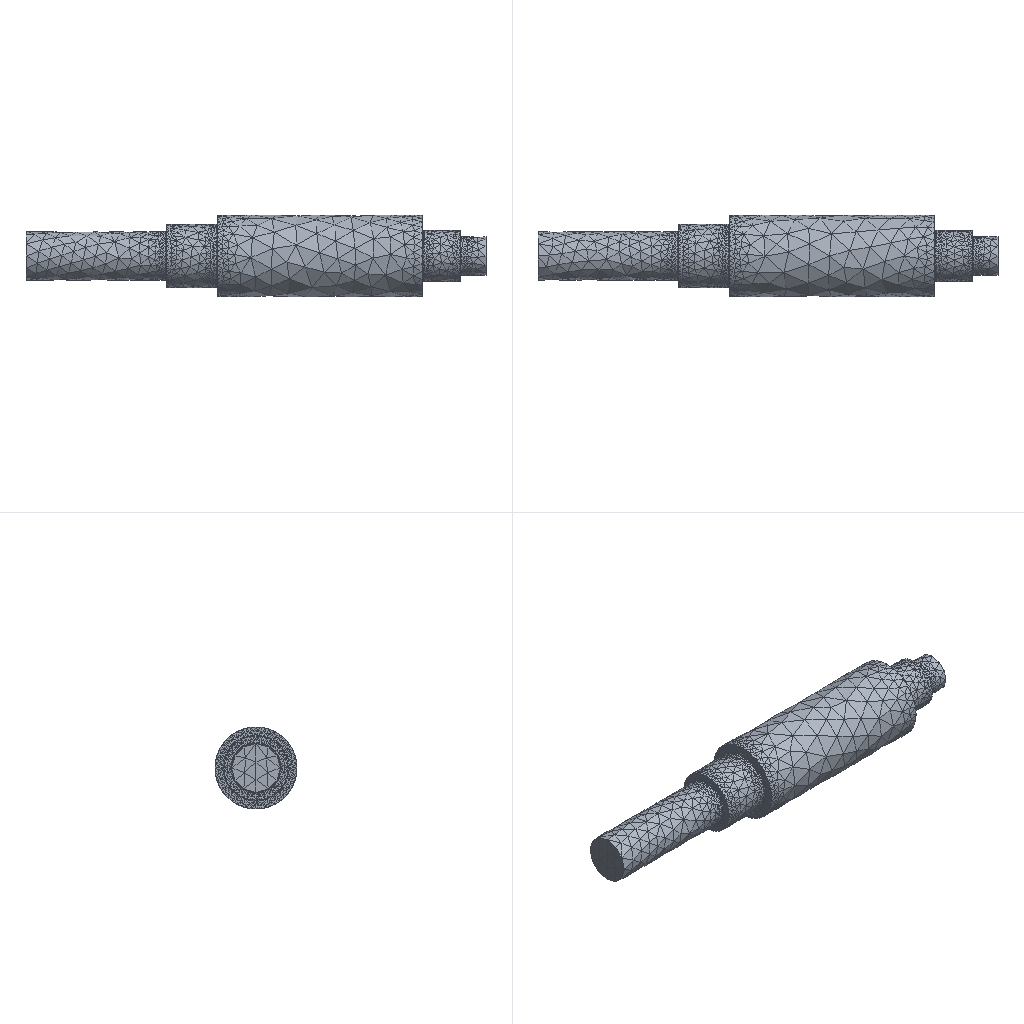Simulation study | ansys workbench
Set-up summary:
category,name,step,type,value,unit,region
solver,ansys_workbench
units,in-lbf-s (psi),,stated,"/units,BIN"
analysis,LS1,,modal,method=lanb; n_modes=20
load_step,LS1,LS1,modal
mesh,nodes,,,91403
mesh,elements,,,61675
element_type,SOLID187,,,61675
material,Structural Steel,,E,2.90075e+07,slinch s^-2 in^-1
material,Structural Steel,,nu,0.3
material,Structural Steel,,density,0.0007345,slinch in^-3
material,Structural Steel,,conductivity,7.556,slinch in s^-3 F^-1
material,Structural Steel,,specific_heat,373723,in^2 s^-2 F^-1
material,Structural Steel,,cte,6.66667e-06,F^-1
material,Structural Steel,,permeability,10000
material,Structural Steel,,resistivity,8.523,ohm cmil in^-1
Ansys APDL input file, long lists of numbers shortened:
/batch
/config,noeldb,1     ! force off writing results to database
*get,_wallstrt,active,,time,wall
! ANSYS input file written by Workbench version 2025 R2
! File used for geometry attach:
/title,wbnew--__ (A5)
! ****** Begin Custom Load Command Snippet ******
/COM, ACT Extensions:
/COM,     LSDYNA, 2025.2
/COM,/COM,     ANSYSMotion, 2025.2
/COM,
! ****** End   Custom Load Command Snippet ******
*DIM,_wb_ProjectScratch_dir,string,248
_wb_ProjectScratch_dir(1) = ''
*DIM,_wb_SolverFiles_dir,string,248
_wb_SolverFiles_dir(1) = ''
*DIM,_wb_userfiles_dir,string,248
_wb_userfiles_dir(1) = ''
/com,--- Data in consistent BIN units. See Solving Units in the help system for more information.
/units,BIN
/nopr
/wb,file,start              !  signify a WB generated input file
/prep7
! Turn off shape checking because checks already performed inside WB mesher.
! See help system for more information.
SHPP,OFF,,NOWARN
/nolist
etcon,set             ! allow ANSYS to choose best KEYOP's for 180x elements, resets any applicable keyopt to MAPDL defaults
/com,*********** Send User Defined Coordinate System(s) ***********
csys,0
/com,*********** Nodes for the whole assembly ***********
nblock,3,,100543
(1i9,3e20.9e3)
        1     0.000000000E+00    -4.580371887E-17    -3.740157480E-01
! (91402 more lines like these left out)
-1
/wb,elem,start            !  set before creation of elements
/com,*********** Elements for Body 1 'Part 1' ***********
et,1,187
MAT,1 $ TYPE,1 $ REAL,1 $ SECNUM,1 $ ESYS,0
eblock,11,COMPACT,,61675
(11i9)
        1     7993    12675     8526     9142    67015    70402    67012    67013    74710    70396
! (61674 more lines like these left out)
-1
secnum,1    ! reset the section ID to default
/wb,elem,end               !  done creating elements
toffst,459.67,      ! Temperature offset from absolute zero
/com,*********** Set Reference Temperature ***********
tref,71.6
/wb,mat,start              !  starting to send materials
/com,*********** Send Materials ***********
Temperature = 'TEMP' ! Temperature
MP,DENS,1,0.0007345,	! slinch in^-3
MP,ALPX,1,6.66666666666667e-06,	! F^-1
MP,C,1,373722.97,	! in^2 s^-2 F^-1
MP,KXX,1,7.556,	! slinch in s^-3 F^-1
MP,RSVX,1,8.523,	! ohm cmil in^-1
MP,EX,1,29007547.543,	! slinch s^-2 in^-1
MP,NUXY,1,0.3,
MP,MURX,1,10000,
/wb,mat,end                !  done sending materials
!************************* Model Summary ********************
!Part 1,	结构钢,	matid,	1
!************************* End Model Summary ********************
! get the diagonal of the bounding box. Needed later for other things
*get,_xmin,node,,mnloc,x
*get,_ymin,node,,mnloc,y
*get,_zmin,node,,mnloc,z
*get,_xmax,node,,mxloc,x
*get,_ymax,node,,mxloc,y
*get,_zmax,node,,mxloc,z
_ASMDIAG=(_xmax-_xmin)*(_xmax-_xmin)+(_ymax-_ymin)*(_ymax-_ymin)+(_zmax-_zmin)*(_zmax-_zmin)
_ASMDIAG=SQRT(_ASMDIAG)
/wb,contact,start          !  starting to send contact
/wb,contact,end            !  done creating contacts
/golist
/wb,load,start             !  starting to send loads
/gst,on,on
fini
*get,_numnode,node,0,count
*get,_numelem,elem,0,count
*get, _MAXELEMNUM, elem, 0, NUM, MAX
*get, _MAXNODENUM, node, 0, NUM, MAX
*get, _MAXELEMTYPE, etyp, 0, NUM, MAX
*get, _MAXREALCONST, rcon, 0, NUM, MAX
/go
/wb,load,end               !  done creating loads
/com,--- Number of total nodes = %_numnode%
/com,--- Number of contact elements = 0
/com,--- Number of spring elements = 0
/com,--- Number of bearing elements = 0
/com,--- Number of solid elements = 61675
/com,--- Number of condensed parts = 0
/com,--- Number of total elements = %_numelem%
*get,_wallbsol,active,,time,wall
/solu
antype,2                   ! modal analysis
_thickRatio=  1     ! Ratio of thick parts in the model
thexpand,off     ! ignore thermal strains
modopt,lanb,20
outres,erase
outres,all,none
outres,nsol,all
outres,strs,all,
outres,epel,all,
outres,eppl,all,
mxpand,,,,yes,,no             ! expand requested element results, but not write them to file.mode
dmpopt,esav,no
dmpopt,emat,no
dmpopt,full,no
! *********** WB SOLVE COMMAND ***********
! check interactive state
*get,ANSINTER_,active,,int
*if,ANSINTER_,ne,0,then
/eof
*endif
solve
/com *************** Write FE CONNECTORS *********
CEWRITE,file,ce,,INTE
*get,_nmodalsolproc,active,0,numcpu
fini
/nopr
*get,_numnode,node,0,count
*get,_numelem,elem,0,count
*get, _MAXELEMNUM, elem, 0, NUM, MAX
*get, _MAXNODENUM, node, 0, NUM, MAX,,,INTERNAL
*get, _MAXELEMTYPE, etyp, 0, NUM, MAX
*get, _MAXREALCONST, rcon, 0, NUM, MAX
*get,_NSOLTHREADS,active,0,ntfs
*get,_NSOLPROCESSES,active,0,npfs
/gopr
*get,_wallasol,active,,time,wall
/post1
/nopr
*dim,_direction,CHAR,6,1
_direction(1) = 'X'
_direction(2) = 'Y'
_direction(3) = 'Z'
_direction(4) = 'ROTX'
_direction(5) = 'ROTY'
_direction(6) = 'ROTZ'
*get,_lastLS,active,0,set,LSTP
*get,_beginset,active,0,set,nset,first,_lastLS
*get,_endset,active,0,set,nset,last,_lastLS
_nummodes = 0
*if,_endset,gt,0,then
_nummodes = _endset - _beginset + 1
*endif
*do,i_mode,1,_nummodes
   *do,j_component,1,6
			*get,PFACT_%i_mode%_%j_component%,MODE,%i_mode%,PFACT,,DIREC,_direction(%j_component%)
   *enddo
*enddo
*dim,_tmdirection,CHAR,6,1
_tmdirection(1) = 'X'
_tmdirection(2) = 'Y'
_tmdirection(3) = 'Z'
_tmdirection(4) = 'X'
_tmdirection(5) = 'Y'
_tmdirection(6) = 'Z'
*do,j_component,1,6
    *if,j_component,gt,3,then
        *get,TOTALMASS_%j_component%,ELEM,0,IOR,_tmdirection(%j_component%)
    *else
        *get,TOTALMASS_%j_component%,ELEM,0,MTOT,_tmdirection(%j_component%)
    *endif
*enddo
/gopr
xmlo,ENCODING,ISO-8859-1
xmlo,parm
/xml,parm,xml
fini
/gopr
*get,_walldone,active,,time,wall
_preptime=(_wallbsol-_wallstrt)*3600
_solvtime=(_wallasol-_wallbsol)*3600
_posttime=(_walldone-_wallasol)*3600
_totaltim=(_walldone-_wallstrt)*3600
*get,_dlbratio,active,0,solu,dlbr
*get,_combtime,active,0,solu,comb
*get,_ssmode,active,0,solu,ssmm
*get,_ndofs,active,0,solu,ndof
/fclean				!clean distributed files
/com,--- Total number of nodes = %_numnode%
/com,--- Total number of elements = %_numelem%
/com,--- Element load balance ratio = %_dlbratio%
/com,--- Time to combine distributed files = %_combtime%
/com,--- Sparse memory mode = %_ssmode%
/com,--- Number of DOF = %_ndofs%
/wb,file,end               ! done with WB generated input
Results summary:
result,analyses[0].index,,,1
result,analyses[0].system,,,SYS
result,analyses[0].deck,,,deck.dat
result,analyses[0].solve_status,,,completed
result,analyses[0].analysis_type,,,modal
result,analyses[0].physics,,,mechanical
result,analyses[0].unit_system,,,"Custom: in, slinch, s, A, degF"
result,analyses[0].n_sets,,,20
result,analyses[0].modal_frequencies_hz[1],,,0
result,analyses[0].modal_frequencies_hz[2],,,0
result,analyses[0].modal_frequencies_hz[3],,,0
result,analyses[0].modal_frequencies_hz[4],,,0.0014
result,analyses[0].modal_frequencies_hz[5],,,0.002551
result,analyses[0].modal_frequencies_hz[6],,,0.002591
result,analyses[0].modal_frequencies_hz[7],,,3938.61
result,analyses[0].modal_frequencies_hz[8],,,3938.64
result,analyses[0].modal_frequencies_hz[9],,,9823.38
result,analyses[0].modal_frequencies_hz[10],,,9823.48
result,analyses[0].modal_frequencies_hz[11],,,11771.7
result,analyses[0].modal_frequencies_hz[12],,,16191.2
result,analyses[0].modal_frequencies_hz[13],,,16191.4
result,analyses[0].modal_frequencies_hz[14],,,16756.5
result,analyses[0].modal_frequencies_hz[15],,,18357.4
result,analyses[0].modal_frequencies_hz[16],,,22471.3
result,analyses[0].modal_frequencies_hz[17],,,22471.6
result,analyses[0].modal_frequencies_hz[18],,,28562.8
result,analyses[0].modal_frequencies_hz[19],,,29857.8
result,analyses[0].modal_frequencies_hz[20],,,29858